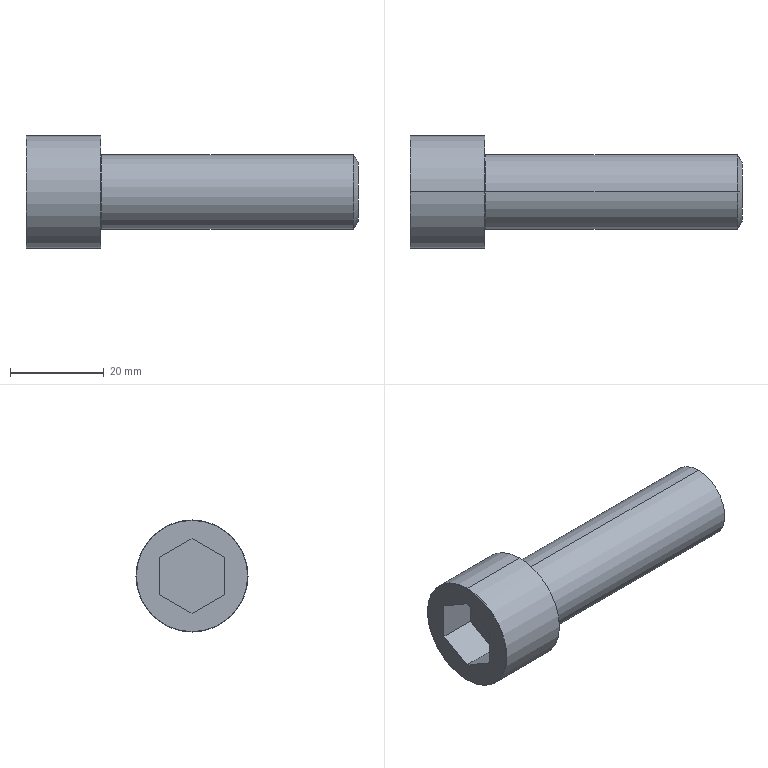Part | SolidWorks | features BlendCut 1, Cut 1, Fillet 1, LPattern 1, RevCut 1, Revolution 1 | 1 solid | 20 faces | box 71 x 24 x 24 mm | volume 16926 mm3 | plane 10 | torus 4 | cylinder 4 | cone 2 | commonest cylinder face diameters 16 x2 24 x2
STEP:
#1=CARTESIAN_POINT('',(0.,0.,11.9));
#2=VERTEX_POINT('',#1);
#3=CARTESIAN_POINT('',(0.,0.,-11.9));
#4=VERTEX_POINT('',#3);
#5=CARTESIAN_POINT('',(0.,0.,0.));
#6=DIRECTION('',(-1.,0.,0.));
#7=DIRECTION('',(0.,0.,-1.));
#8=AXIS2_PLACEMENT_3D('',#5,#6,#7);
#9=CIRCLE('',#8,11.9);
#10=EDGE_CURVE('',#2,#4,#9,.T.);
#11=ORIENTED_EDGE('',*,*,#10,.F.);
#12=CARTESIAN_POINT('',(0.1,0.,12.));
#13=VERTEX_POINT('',#12);
#14=CARTESIAN_POINT('',(0.1,0.,11.9));
#15=DIRECTION('',(0.,1.,0.));
#16=DIRECTION('',(0.,0.,1.));
#17=AXIS2_PLACEMENT_3D('',#14,#15,#16);
#18=CIRCLE('',#17,0.1);
#19=EDGE_CURVE('',#2,#13,#18,.T.);
#20=ORIENTED_EDGE('',*,*,#19,.T.);
#21=CARTESIAN_POINT('',(0.1,0.,-12.));
#22=VERTEX_POINT('',#21);
#23=CARTESIAN_POINT('',(0.1,0.,0.));
#24=DIRECTION('',(1.,0.,0.));
#25=DIRECTION('',(0.,0.,-1.));
#26=AXIS2_PLACEMENT_3D('',#23,#24,#25);
#27=CIRCLE('',#26,12.);
#28=EDGE_CURVE('',#22,#13,#27,.T.);
#29=ORIENTED_EDGE('',*,*,#28,.F.);
#30=CARTESIAN_POINT('',(0.1,0.,-11.9));
#31=DIRECTION('',(0.,-1.,0.));
#32=DIRECTION('',(0.,0.,-1.));
#33=AXIS2_PLACEMENT_3D('',#30,#31,#32);
#34=CIRCLE('',#33,0.1);
#35=EDGE_CURVE('',#4,#22,#34,.T.);
#36=ORIENTED_EDGE('',*,*,#35,.F.);
#37=EDGE_LOOP('',(#11,#20,#29,#36));
#38=FACE_OUTER_BOUND('',#37,.T.);
#39=CARTESIAN_POINT('',(0.1,0.,0.));
#40=DIRECTION('',(1.,0.,0.));
#41=DIRECTION('',(0.,0.,-1.));
#42=AXIS2_PLACEMENT_3D('',#39,#40,#41);
#43=TOROIDAL_SURFACE('',#42,11.9,0.1);
#44=ADVANCED_FACE('',(#38),#43,.T.);
#45=CARTESIAN_POINT('',(71.,0.,6.268));
#46=VERTEX_POINT('',#45);
#47=CARTESIAN_POINT('',(71.,0.,-6.268));
#48=VERTEX_POINT('',#47);
#49=CARTESIAN_POINT('',(71.,0.,0.));
#50=DIRECTION('',(-1.,0.,0.));
#51=DIRECTION('',(0.,0.,1.));
#52=AXIS2_PLACEMENT_3D('',#49,#50,#51);
#53=CIRCLE('',#52,6.268);
#54=EDGE_CURVE('',#46,#48,#53,.T.);
#55=ORIENTED_EDGE('',*,*,#54,.T.);
#56=CARTESIAN_POINT('',(70.,0.,-8.));
#57=VERTEX_POINT('',#56);
#58=CARTESIAN_POINT('',(70.,0.,-8.));
#59=DIRECTION('',(-0.5,0.,-0.866));
#60=VECTOR('',#59,1000.);
#61=LINE('',#58,#60);
#62=EDGE_CURVE('',#48,#57,#61,.T.);
#63=ORIENTED_EDGE('',*,*,#62,.T.);
#64=CARTESIAN_POINT('',(70.,0.,8.));
#65=VERTEX_POINT('',#64);
#66=CARTESIAN_POINT('',(70.,0.,0.));
#67=DIRECTION('',(-1.,0.,0.));
#68=DIRECTION('',(0.,0.,1.));
#69=AXIS2_PLACEMENT_3D('',#66,#67,#68);
#70=CIRCLE('',#69,8.);
#71=EDGE_CURVE('',#65,#57,#70,.T.);
#72=ORIENTED_EDGE('',*,*,#71,.F.);
#73=CARTESIAN_POINT('',(70.,0.,8.));
#74=DIRECTION('',(-0.5,0.,0.866));
#75=VECTOR('',#74,1000.);
#76=LINE('',#73,#75);
#77=EDGE_CURVE('',#46,#65,#76,.T.);
#78=ORIENTED_EDGE('',*,*,#77,.F.);
#79=EDGE_LOOP('',(#55,#63,#72,#78));
#80=FACE_OUTER_BOUND('',#79,.T.);
#81=CARTESIAN_POINT('',(70.,0.,0.));
#82=DIRECTION('',(-1.,0.,0.));
#83=DIRECTION('',(0.,0.,1.));
#84=AXIS2_PLACEMENT_3D('',#81,#82,#83);
#85=CONICAL_SURFACE('',#84,8.,1.047);
#86=ADVANCED_FACE('',(#80),#85,.T.);
#87=CARTESIAN_POINT('',(16.,0.,-8.2));
#88=VERTEX_POINT('',#87);
#89=CARTESIAN_POINT('',(16.,0.,8.2));
#90=VERTEX_POINT('',#89);
#91=CARTESIAN_POINT('',(16.,0.,0.));
#92=DIRECTION('',(-1.,0.,0.));
#93=DIRECTION('',(0.,0.,1.));
#94=AXIS2_PLACEMENT_3D('',#91,#92,#93);
#95=CIRCLE('',#94,8.2);
#96=EDGE_CURVE('',#88,#90,#95,.T.);
#97=ORIENTED_EDGE('',*,*,#96,.F.);
#98=CARTESIAN_POINT('',(16.2,0.,-8.));
#99=VERTEX_POINT('',#98);
#100=CARTESIAN_POINT('',(16.2,0.,-8.2));
#101=DIRECTION('',(0.,1.,0.));
#102=DIRECTION('',(0.,0.,1.));
#103=AXIS2_PLACEMENT_3D('',#100,#101,#102);
#104=CIRCLE('',#103,0.2);
#105=EDGE_CURVE('',#88,#99,#104,.T.);
#106=ORIENTED_EDGE('',*,*,#105,.T.);
#107=CARTESIAN_POINT('',(16.2,0.,8.));
#108=VERTEX_POINT('',#107);
#109=CARTESIAN_POINT('',(16.2,0.,0.));
#110=DIRECTION('',(-1.,0.,0.));
#111=DIRECTION('',(0.,0.,1.));
#112=AXIS2_PLACEMENT_3D('',#109,#110,#111);
#113=CIRCLE('',#112,8.);
#114=EDGE_CURVE('',#99,#108,#113,.T.);
#115=ORIENTED_EDGE('',*,*,#114,.T.);
#116=CARTESIAN_POINT('',(16.2,0.,8.2));
#117=DIRECTION('',(0.,-1.,0.));
#118=DIRECTION('',(0.,0.,-1.));
#119=AXIS2_PLACEMENT_3D('',#116,#117,#118);
#120=CIRCLE('',#119,0.2);
#121=EDGE_CURVE('',#90,#108,#120,.T.);
#122=ORIENTED_EDGE('',*,*,#121,.F.);
#123=EDGE_LOOP('',(#97,#106,#115,#122));
#124=FACE_OUTER_BOUND('',#123,.T.);
#125=CARTESIAN_POINT('',(16.2,0.,0.));
#126=DIRECTION('',(-1.,0.,0.));
#127=DIRECTION('',(0.,0.,1.));
#128=AXIS2_PLACEMENT_3D('',#125,#126,#127);
#129=TOROIDAL_SURFACE('',#128,8.2,0.2);
#130=ADVANCED_FACE('',(#124),#129,.F.);
#131=CARTESIAN_POINT('',(16.,0.,12.));
#132=VERTEX_POINT('',#131);
#133=CARTESIAN_POINT('',(16.,0.,-12.));
#134=VERTEX_POINT('',#133);
#135=CARTESIAN_POINT('',(16.,0.,0.));
#136=DIRECTION('',(-1.,0.,0.));
#137=DIRECTION('',(0.,0.,1.));
#138=AXIS2_PLACEMENT_3D('',#135,#136,#137);
#139=CIRCLE('',#138,12.);
#140=EDGE_CURVE('',#132,#134,#139,.T.);
#141=ORIENTED_EDGE('',*,*,#140,.T.);
#142=CARTESIAN_POINT('',(0.,0.,-12.));
#143=DIRECTION('',(-1.,0.,0.));
#144=VECTOR('',#143,1000.);
#145=LINE('',#142,#144);
#146=EDGE_CURVE('',#134,#22,#145,.T.);
#147=ORIENTED_EDGE('',*,*,#146,.T.);
#148=ORIENTED_EDGE('',*,*,#28,.T.);
#149=CARTESIAN_POINT('',(0.,0.,12.));
#150=DIRECTION('',(-1.,0.,0.));
#151=VECTOR('',#150,1000.);
#152=LINE('',#149,#151);
#153=EDGE_CURVE('',#132,#13,#152,.T.);
#154=ORIENTED_EDGE('',*,*,#153,.F.);
#155=EDGE_LOOP('',(#141,#147,#148,#154));
#156=FACE_OUTER_BOUND('',#155,.T.);
#157=CARTESIAN_POINT('',(0.,0.,0.));
#158=DIRECTION('',(-1.,0.,0.));
#159=DIRECTION('',(0.,0.,1.));
#160=AXIS2_PLACEMENT_3D('',#157,#158,#159);
#161=CYLINDRICAL_SURFACE('',#160,12.);
#162=ADVANCED_FACE('',(#156),#161,.T.);
#163=ORIENTED_EDGE('',*,*,#71,.T.);
#164=CARTESIAN_POINT('',(0.,0.,-8.));
#165=DIRECTION('',(-1.,0.,0.));
#166=VECTOR('',#165,1000.);
#167=LINE('',#164,#166);
#168=EDGE_CURVE('',#57,#99,#167,.T.);
#169=ORIENTED_EDGE('',*,*,#168,.T.);
#170=CARTESIAN_POINT('',(16.2,0.,0.));
#171=DIRECTION('',(-1.,0.,0.));
#172=DIRECTION('',(0.,0.,1.));
#173=AXIS2_PLACEMENT_3D('',#170,#171,#172);
#174=CIRCLE('',#173,8.);
#175=EDGE_CURVE('',#108,#99,#174,.T.);
#176=ORIENTED_EDGE('',*,*,#175,.F.);
#177=CARTESIAN_POINT('',(0.,0.,8.));
#178=DIRECTION('',(-1.,0.,0.));
#179=VECTOR('',#178,1000.);
#180=LINE('',#177,#179);
#181=EDGE_CURVE('',#65,#108,#180,.T.);
#182=ORIENTED_EDGE('',*,*,#181,.F.);
#183=EDGE_LOOP('',(#163,#169,#176,#182));
#184=FACE_OUTER_BOUND('',#183,.T.);
#185=CARTESIAN_POINT('',(0.,0.,0.));
#186=DIRECTION('',(-1.,0.,0.));
#187=DIRECTION('',(0.,0.,1.));
#188=AXIS2_PLACEMENT_3D('',#185,#186,#187);
#189=CYLINDRICAL_SURFACE('',#188,8.);
#190=ADVANCED_FACE('',(#184),#189,.T.);
#191=ORIENTED_EDGE('',*,*,#168,.F.);
#192=CARTESIAN_POINT('',(70.,0.,0.));
#193=DIRECTION('',(-1.,0.,0.));
#194=DIRECTION('',(0.,0.,1.));
#195=AXIS2_PLACEMENT_3D('',#192,#193,#194);
#196=CIRCLE('',#195,8.);
#197=EDGE_CURVE('',#57,#65,#196,.T.);
#198=ORIENTED_EDGE('',*,*,#197,.T.);
#199=ORIENTED_EDGE('',*,*,#181,.T.);
#200=ORIENTED_EDGE('',*,*,#114,.F.);
#201=EDGE_LOOP('',(#191,#198,#199,#200));
#202=FACE_OUTER_BOUND('',#201,.T.);
#203=CARTESIAN_POINT('',(0.,0.,0.));
#204=DIRECTION('',(-1.,0.,0.));
#205=DIRECTION('',(0.,0.,1.));
#206=AXIS2_PLACEMENT_3D('',#203,#204,#205);
#207=CYLINDRICAL_SURFACE('',#206,8.);
#208=ADVANCED_FACE('',(#202),#207,.T.);
#209=CARTESIAN_POINT('',(0.,0.,0.));
#210=DIRECTION('',(-1.,0.,0.));
#211=DIRECTION('',(0.,0.,-1.));
#212=AXIS2_PLACEMENT_3D('',#209,#210,#211);
#213=CIRCLE('',#212,11.9);
#214=EDGE_CURVE('',#4,#2,#213,.T.);
#215=ORIENTED_EDGE('',*,*,#214,.T.);
#216=ORIENTED_EDGE('',*,*,#10,.T.);
#217=EDGE_LOOP('',(#215,#216));
#218=FACE_OUTER_BOUND('',#217,.T.);
#219=CARTESIAN_POINT('',(0.,0.,8.));
#220=VERTEX_POINT('',#219);
#221=CARTESIAN_POINT('',(0.,6.928,4.));
#222=VERTEX_POINT('',#221);
#223=CARTESIAN_POINT('',(0.,0.,8.));
#224=DIRECTION('',(0.,0.866,-0.5));
#225=VECTOR('',#224,1000.);
#226=LINE('',#223,#225);
#227=EDGE_CURVE('',#220,#222,#226,.T.);
#228=ORIENTED_EDGE('',*,*,#227,.F.);
#229=CARTESIAN_POINT('',(0.,-6.928,4.));
#230=VERTEX_POINT('',#229);
#231=CARTESIAN_POINT('',(0.,-6.928,4.));
#232=DIRECTION('',(0.,0.866,0.5));
#233=VECTOR('',#232,1000.);
#234=LINE('',#231,#233);
#235=EDGE_CURVE('',#230,#220,#234,.T.);
#236=ORIENTED_EDGE('',*,*,#235,.F.);
#237=CARTESIAN_POINT('',(0.,-6.928,-4.));
#238=VERTEX_POINT('',#237);
#239=CARTESIAN_POINT('',(0.,-6.928,-4.));
#240=DIRECTION('',(0.,0.,1.));
#241=VECTOR('',#240,1000.);
#242=LINE('',#239,#241);
#243=EDGE_CURVE('',#238,#230,#242,.T.);
#244=ORIENTED_EDGE('',*,*,#243,.F.);
#245=CARTESIAN_POINT('',(0.,0.,-8.));
#246=VERTEX_POINT('',#245);
#247=CARTESIAN_POINT('',(0.,0.,-8.));
#248=DIRECTION('',(0.,-0.866,0.5));
#249=VECTOR('',#248,1000.);
#250=LINE('',#247,#249);
#251=EDGE_CURVE('',#246,#238,#250,.T.);
#252=ORIENTED_EDGE('',*,*,#251,.F.);
#253=CARTESIAN_POINT('',(0.,6.928,-4.));
#254=VERTEX_POINT('',#253);
#255=CARTESIAN_POINT('',(0.,6.928,-4.));
#256=DIRECTION('',(0.,-0.866,-0.5));
#257=VECTOR('',#256,1000.);
#258=LINE('',#255,#257);
#259=EDGE_CURVE('',#254,#246,#258,.T.);
#260=ORIENTED_EDGE('',*,*,#259,.F.);
#261=CARTESIAN_POINT('',(0.,6.928,4.));
#262=DIRECTION('',(0.,0.,-1.));
#263=VECTOR('',#262,1000.);
#264=LINE('',#261,#263);
#265=EDGE_CURVE('',#222,#254,#264,.T.);
#266=ORIENTED_EDGE('',*,*,#265,.F.);
#267=EDGE_LOOP('',(#228,#236,#244,#252,#260,#266));
#268=FACE_BOUND('',#267,.T.);
#269=CARTESIAN_POINT('',(0.,0.,0.));
#270=DIRECTION('',(1.,0.,0.));
#271=DIRECTION('',(0.,0.,-1.));
#272=AXIS2_PLACEMENT_3D('',#269,#270,#271);
#273=PLANE('',#272);
#274=ADVANCED_FACE('',(#218,#268),#273,.F.);
#275=ORIENTED_EDGE('',*,*,#146,.F.);
#276=CARTESIAN_POINT('',(16.,0.,0.));
#277=DIRECTION('',(-1.,0.,0.));
#278=DIRECTION('',(0.,0.,1.));
#279=AXIS2_PLACEMENT_3D('',#276,#277,#278);
#280=CIRCLE('',#279,12.);
#281=EDGE_CURVE('',#134,#132,#280,.T.);
#282=ORIENTED_EDGE('',*,*,#281,.T.);
#283=ORIENTED_EDGE('',*,*,#153,.T.);
#284=CARTESIAN_POINT('',(0.1,0.,0.));
#285=DIRECTION('',(1.,0.,0.));
#286=DIRECTION('',(0.,0.,-1.));
#287=AXIS2_PLACEMENT_3D('',#284,#285,#286);
#288=CIRCLE('',#287,12.);
#289=EDGE_CURVE('',#13,#22,#288,.T.);
#290=ORIENTED_EDGE('',*,*,#289,.T.);
#291=EDGE_LOOP('',(#275,#282,#283,#290));
#292=FACE_OUTER_BOUND('',#291,.T.);
#293=CARTESIAN_POINT('',(0.,0.,0.));
#294=DIRECTION('',(-1.,0.,0.));
#295=DIRECTION('',(0.,0.,1.));
#296=AXIS2_PLACEMENT_3D('',#293,#294,#295);
#297=CYLINDRICAL_SURFACE('',#296,12.);
#298=ADVANCED_FACE('',(#292),#297,.T.);
#299=ORIENTED_EDGE('',*,*,#140,.F.);
#300=ORIENTED_EDGE('',*,*,#281,.F.);
#301=EDGE_LOOP('',(#299,#300));
#302=FACE_OUTER_BOUND('',#301,.T.);
#303=CARTESIAN_POINT('',(16.,0.,0.));
#304=DIRECTION('',(-1.,0.,0.));
#305=DIRECTION('',(0.,0.,1.));
#306=AXIS2_PLACEMENT_3D('',#303,#304,#305);
#307=CIRCLE('',#306,8.2);
#308=EDGE_CURVE('',#90,#88,#307,.T.);
#309=ORIENTED_EDGE('',*,*,#308,.T.);
#310=ORIENTED_EDGE('',*,*,#96,.T.);
#311=EDGE_LOOP('',(#309,#310));
#312=FACE_BOUND('',#311,.T.);
#313=CARTESIAN_POINT('',(16.,12.,0.));
#314=DIRECTION('',(-1.,0.,0.));
#315=DIRECTION('',(0.,0.,1.));
#316=AXIS2_PLACEMENT_3D('',#313,#314,#315);
#317=PLANE('',#316);
#318=ADVANCED_FACE('',(#302,#312),#317,.F.);
#319=ORIENTED_EDGE('',*,*,#105,.F.);
#320=ORIENTED_EDGE('',*,*,#308,.F.);
#321=ORIENTED_EDGE('',*,*,#121,.T.);
#322=ORIENTED_EDGE('',*,*,#175,.T.);
#323=EDGE_LOOP('',(#319,#320,#321,#322));
#324=FACE_OUTER_BOUND('',#323,.T.);
#325=CARTESIAN_POINT('',(16.2,0.,0.));
#326=DIRECTION('',(-1.,0.,0.));
#327=DIRECTION('',(0.,0.,1.));
#328=AXIS2_PLACEMENT_3D('',#325,#326,#327);
#329=TOROIDAL_SURFACE('',#328,8.2,0.2);
#330=ADVANCED_FACE('',(#324),#329,.F.);
#331=ORIENTED_EDGE('',*,*,#235,.T.);
#332=CARTESIAN_POINT('',(8.,0.,8.));
#333=VERTEX_POINT('',#332);
#334=CARTESIAN_POINT('',(8.,0.,8.));
#335=DIRECTION('',(-1.,0.,0.));
#336=VECTOR('',#335,1000.);
#337=LINE('',#334,#336);
#338=EDGE_CURVE('',#333,#220,#337,.T.);
#339=ORIENTED_EDGE('',*,*,#338,.F.);
#340=CARTESIAN_POINT('',(8.,-6.928,4.));
#341=VERTEX_POINT('',#340);
#342=CARTESIAN_POINT('',(8.,-6.928,4.));
#343=DIRECTION('',(0.,0.866,0.5));
#344=VECTOR('',#343,1000.);
#345=LINE('',#342,#344);
#346=EDGE_CURVE('',#341,#333,#345,.T.);
#347=ORIENTED_EDGE('',*,*,#346,.F.);
#348=CARTESIAN_POINT('',(8.,-6.928,4.));
#349=DIRECTION('',(-1.,0.,0.));
#350=VECTOR('',#349,1000.);
#351=LINE('',#348,#350);
#352=EDGE_CURVE('',#341,#230,#351,.T.);
#353=ORIENTED_EDGE('',*,*,#352,.T.);
#354=EDGE_LOOP('',(#331,#339,#347,#353));
#355=FACE_OUTER_BOUND('',#354,.T.);
#356=CARTESIAN_POINT('',(8.,-6.928,4.));
#357=DIRECTION('',(0.,-0.5,0.866));
#358=DIRECTION('',(0.,-0.866,-0.5));
#359=AXIS2_PLACEMENT_3D('',#356,#357,#358);
#360=PLANE('',#359);
#361=ADVANCED_FACE('',(#355),#360,.F.);
#362=ORIENTED_EDGE('',*,*,#243,.T.);
#363=ORIENTED_EDGE('',*,*,#352,.F.);
#364=CARTESIAN_POINT('',(8.,-6.928,-4.));
#365=VERTEX_POINT('',#364);
#366=CARTESIAN_POINT('',(8.,-6.928,-4.));
#367=DIRECTION('',(0.,0.,1.));
#368=VECTOR('',#367,1000.);
#369=LINE('',#366,#368);
#370=EDGE_CURVE('',#365,#341,#369,.T.);
#371=ORIENTED_EDGE('',*,*,#370,.F.);
#372=CARTESIAN_POINT('',(8.,-6.928,-4.));
#373=DIRECTION('',(-1.,0.,0.));
#374=VECTOR('',#373,1000.);
#375=LINE('',#372,#374);
#376=EDGE_CURVE('',#365,#238,#375,.T.);
#377=ORIENTED_EDGE('',*,*,#376,.T.);
#378=EDGE_LOOP('',(#362,#363,#371,#377));
#379=FACE_OUTER_BOUND('',#378,.T.);
#380=CARTESIAN_POINT('',(8.,-6.928,-4.));
#381=DIRECTION('',(0.,-1.,0.));
#382=DIRECTION('',(0.,0.,-1.));
#383=AXIS2_PLACEMENT_3D('',#380,#381,#382);
#384=PLANE('',#383);
#385=ADVANCED_FACE('',(#379),#384,.F.);
#386=ORIENTED_EDGE('',*,*,#251,.T.);
#387=ORIENTED_EDGE('',*,*,#376,.F.);
#388=CARTESIAN_POINT('',(8.,0.,-8.));
#389=VERTEX_POINT('',#388);
#390=CARTESIAN_POINT('',(8.,0.,-8.));
#391=DIRECTION('',(0.,-0.866,0.5));
#392=VECTOR('',#391,1000.);
#393=LINE('',#390,#392);
#394=EDGE_CURVE('',#389,#365,#393,.T.);
#395=ORIENTED_EDGE('',*,*,#394,.F.);
#396=CARTESIAN_POINT('',(8.,0.,-8.));
#397=DIRECTION('',(-1.,0.,0.));
#398=VECTOR('',#397,1000.);
#399=LINE('',#396,#398);
#400=EDGE_CURVE('',#389,#246,#399,.T.);
#401=ORIENTED_EDGE('',*,*,#400,.T.);
#402=EDGE_LOOP('',(#386,#387,#395,#401));
#403=FACE_OUTER_BOUND('',#402,.T.);
#404=CARTESIAN_POINT('',(8.,0.,-8.));
#405=DIRECTION('',(0.,-0.5,-0.866));
#406=DIRECTION('',(0.,0.866,-0.5));
#407=AXIS2_PLACEMENT_3D('',#404,#405,#406);
#408=PLANE('',#407);
#409=ADVANCED_FACE('',(#403),#408,.F.);
#410=ORIENTED_EDGE('',*,*,#259,.T.);
#411=ORIENTED_EDGE('',*,*,#400,.F.);
#412=CARTESIAN_POINT('',(8.,6.928,-4.));
#413=VERTEX_POINT('',#412);
#414=CARTESIAN_POINT('',(8.,6.928,-4.));
#415=DIRECTION('',(0.,-0.866,-0.5));
#416=VECTOR('',#415,1000.);
#417=LINE('',#414,#416);
#418=EDGE_CURVE('',#413,#389,#417,.T.);
#419=ORIENTED_EDGE('',*,*,#418,.F.);
#420=CARTESIAN_POINT('',(8.,6.928,-4.));
#421=DIRECTION('',(-1.,0.,0.));
#422=VECTOR('',#421,1000.);
#423=LINE('',#420,#422);
#424=EDGE_CURVE('',#413,#254,#423,.T.);
#425=ORIENTED_EDGE('',*,*,#424,.T.);
#426=EDGE_LOOP('',(#410,#411,#419,#425));
#427=FACE_OUTER_BOUND('',#426,.T.);
#428=CARTESIAN_POINT('',(8.,6.928,-4.));
#429=DIRECTION('',(0.,0.5,-0.866));
#430=DIRECTION('',(0.,0.866,0.5));
#431=AXIS2_PLACEMENT_3D('',#428,#429,#430);
#432=PLANE('',#431);
#433=ADVANCED_FACE('',(#427),#432,.F.);
#434=ORIENTED_EDGE('',*,*,#265,.T.);
#435=ORIENTED_EDGE('',*,*,#424,.F.);
#436=CARTESIAN_POINT('',(8.,6.928,4.));
#437=VERTEX_POINT('',#436);
#438=CARTESIAN_POINT('',(8.,6.928,4.));
#439=DIRECTION('',(0.,0.,-1.));
#440=VECTOR('',#439,1000.);
#441=LINE('',#438,#440);
#442=EDGE_CURVE('',#437,#413,#441,.T.);
#443=ORIENTED_EDGE('',*,*,#442,.F.);
#444=CARTESIAN_POINT('',(8.,6.928,4.));
#445=DIRECTION('',(-1.,0.,0.));
#446=VECTOR('',#445,1000.);
#447=LINE('',#444,#446);
#448=EDGE_CURVE('',#437,#222,#447,.T.);
#449=ORIENTED_EDGE('',*,*,#448,.T.);
#450=EDGE_LOOP('',(#434,#435,#443,#449));
#451=FACE_OUTER_BOUND('',#450,.T.);
#452=CARTESIAN_POINT('',(8.,6.928,4.));
#453=DIRECTION('',(0.,1.,0.));
#454=DIRECTION('',(0.,0.,1.));
#455=AXIS2_PLACEMENT_3D('',#452,#453,#454);
#456=PLANE('',#455);
#457=ADVANCED_FACE('',(#451),#456,.F.);
#458=ORIENTED_EDGE('',*,*,#227,.T.);
#459=ORIENTED_EDGE('',*,*,#448,.F.);
#460=CARTESIAN_POINT('',(8.,0.,8.));
#461=DIRECTION('',(0.,0.866,-0.5));
#462=VECTOR('',#461,1000.);
#463=LINE('',#460,#462);
#464=EDGE_CURVE('',#333,#437,#463,.T.);
#465=ORIENTED_EDGE('',*,*,#464,.F.);
#466=ORIENTED_EDGE('',*,*,#338,.T.);
#467=EDGE_LOOP('',(#458,#459,#465,#466));
#468=FACE_OUTER_BOUND('',#467,.T.);
#469=CARTESIAN_POINT('',(8.,0.,8.));
#470=DIRECTION('',(0.,0.5,0.866));
#471=DIRECTION('',(0.,-0.866,0.5));
#472=AXIS2_PLACEMENT_3D('',#469,#470,#471);
#473=PLANE('',#472);
#474=ADVANCED_FACE('',(#468),#473,.F.);
#475=ORIENTED_EDGE('',*,*,#346,.T.);
#476=ORIENTED_EDGE('',*,*,#464,.T.);
#477=ORIENTED_EDGE('',*,*,#442,.T.);
#478=ORIENTED_EDGE('',*,*,#418,.T.);
#479=ORIENTED_EDGE('',*,*,#394,.T.);
#480=ORIENTED_EDGE('',*,*,#370,.T.);
#481=EDGE_LOOP('',(#475,#476,#477,#478,#479,#480));
#482=FACE_OUTER_BOUND('',#481,.T.);
#483=CARTESIAN_POINT('',(8.,-6.928,4.));
#484=DIRECTION('',(1.,0.,0.));
#485=DIRECTION('',(0.,0.,-1.));
#486=AXIS2_PLACEMENT_3D('',#483,#484,#485);
#487=PLANE('',#486);
#488=ADVANCED_FACE('',(#482),#487,.F.);
#489=ORIENTED_EDGE('',*,*,#62,.F.);
#490=CARTESIAN_POINT('',(71.,0.,0.));
#491=DIRECTION('',(-1.,0.,0.));
#492=DIRECTION('',(0.,0.,1.));
#493=AXIS2_PLACEMENT_3D('',#490,#491,#492);
#494=CIRCLE('',#493,6.268);
#495=EDGE_CURVE('',#48,#46,#494,.T.);
#496=ORIENTED_EDGE('',*,*,#495,.T.);
#497=ORIENTED_EDGE('',*,*,#77,.T.);
#498=ORIENTED_EDGE('',*,*,#197,.F.);
#499=EDGE_LOOP('',(#489,#496,#497,#498));
#500=FACE_OUTER_BOUND('',#499,.T.);
#501=CARTESIAN_POINT('',(70.,0.,0.));
#502=DIRECTION('',(-1.,0.,0.));
#503=DIRECTION('',(0.,0.,1.));
#504=AXIS2_PLACEMENT_3D('',#501,#502,#503);
#505=CONICAL_SURFACE('',#504,8.,1.047);
#506=ADVANCED_FACE('',(#500),#505,.T.);
#507=ORIENTED_EDGE('',*,*,#54,.F.);
#508=ORIENTED_EDGE('',*,*,#495,.F.);
#509=EDGE_LOOP('',(#507,#508));
#510=FACE_OUTER_BOUND('',#509,.T.);
#511=CARTESIAN_POINT('',(71.,8.,0.));
#512=DIRECTION('',(-1.,0.,0.));
#513=DIRECTION('',(0.,0.,1.));
#514=AXIS2_PLACEMENT_3D('',#511,#512,#513);
#515=PLANE('',#514);
#516=ADVANCED_FACE('',(#510),#515,.F.);
#517=ORIENTED_EDGE('',*,*,#19,.F.);
#518=ORIENTED_EDGE('',*,*,#214,.F.);
#519=ORIENTED_EDGE('',*,*,#35,.T.);
#520=ORIENTED_EDGE('',*,*,#289,.F.);
#521=EDGE_LOOP('',(#517,#518,#519,#520));
#522=FACE_OUTER_BOUND('',#521,.T.);
#523=CARTESIAN_POINT('',(0.1,0.,0.));
#524=DIRECTION('',(1.,0.,0.));
#525=DIRECTION('',(0.,0.,-1.));
#526=AXIS2_PLACEMENT_3D('',#523,#524,#525);
#527=TOROIDAL_SURFACE('',#526,11.9,0.1);
#528=ADVANCED_FACE('',(#522),#527,.T.);
#529=CLOSED_SHELL('',(#44,#86,#130,#162,#190,#208,#274,#298,#318,#330,#361,#385,#409,#433,#457,#474,#488,#506,#516,#528));
#530=MANIFOLD_SOLID_BREP('',#529);
#531=CARTESIAN_POINT('',(0.,0.,0.));
#532=DIRECTION('',(0.,0.,1.));
#533=DIRECTION('',(1.,0.,0.));
#534=AXIS2_PLACEMENT_3D('',#531,#532,#533);
#535=(LENGTH_UNIT()NAMED_UNIT(*)SI_UNIT(.MILLI.,.METRE.));
#536=UNCERTAINTY_MEASURE_WITH_UNIT(LENGTH_MEASURE(0.00001),#535,'','');
#537=(NAMED_UNIT(*)PLANE_ANGLE_UNIT()SI_UNIT($,.RADIAN.));
#538=(NAMED_UNIT(*)SI_UNIT($,.STERADIAN.)SOLID_ANGLE_UNIT());
#539=(GEOMETRIC_REPRESENTATION_CONTEXT(3)GLOBAL_UNCERTAINTY_ASSIGNED_CONTEXT((#536))GLOBAL_UNIT_ASSIGNED_CONTEXT((#535,#537,#538))REPRESENTATION_CONTEXT('',''));
#540=ADVANCED_BREP_SHAPE_REPRESENTATION('',(#530,#534),#539);